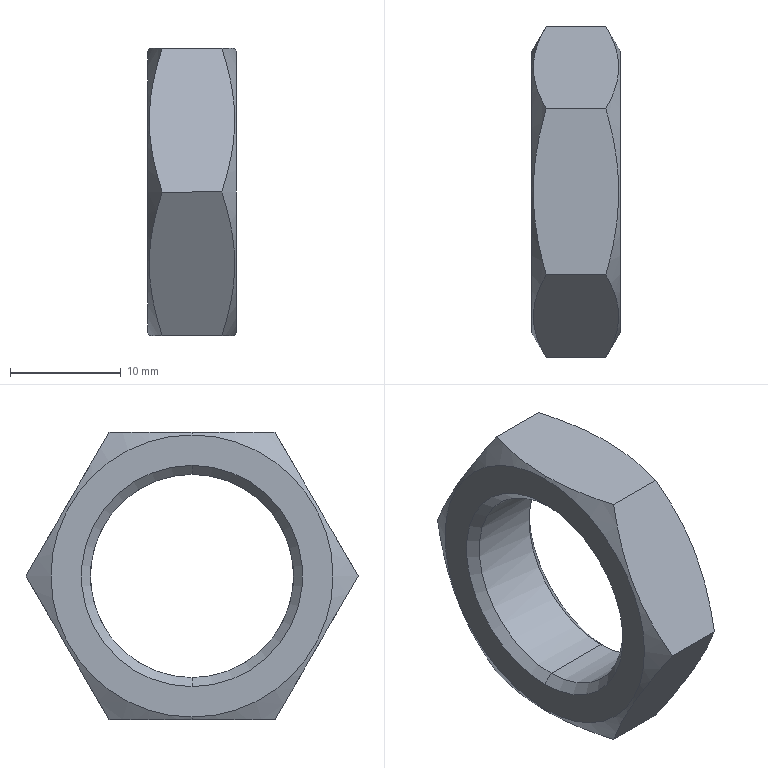Part | STEP file | _CM2_SN-020B(20) | 1 solid | 18 faces | box 8 x 30.022 x 26 mm | volume 2466 mm3 | cone 8 | plane 8 | cylinder 2 | commonest cylinder face diameters 18.376 x2